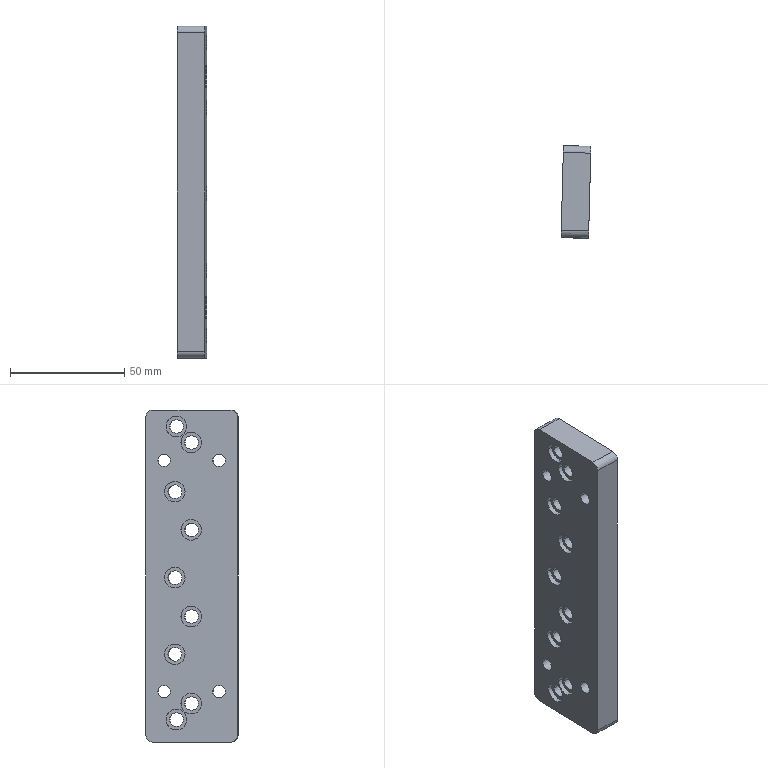Part | STEP file | 333 | 1 solid | 75 faces | box 13.043 x 40.3 x 145 mm | volume 63615 mm3 | cylinder 56 | plane 19 | commonest cylinder face diameters 6.03 x18 9 x18 5.5 x8 9.5 x8 6 x4